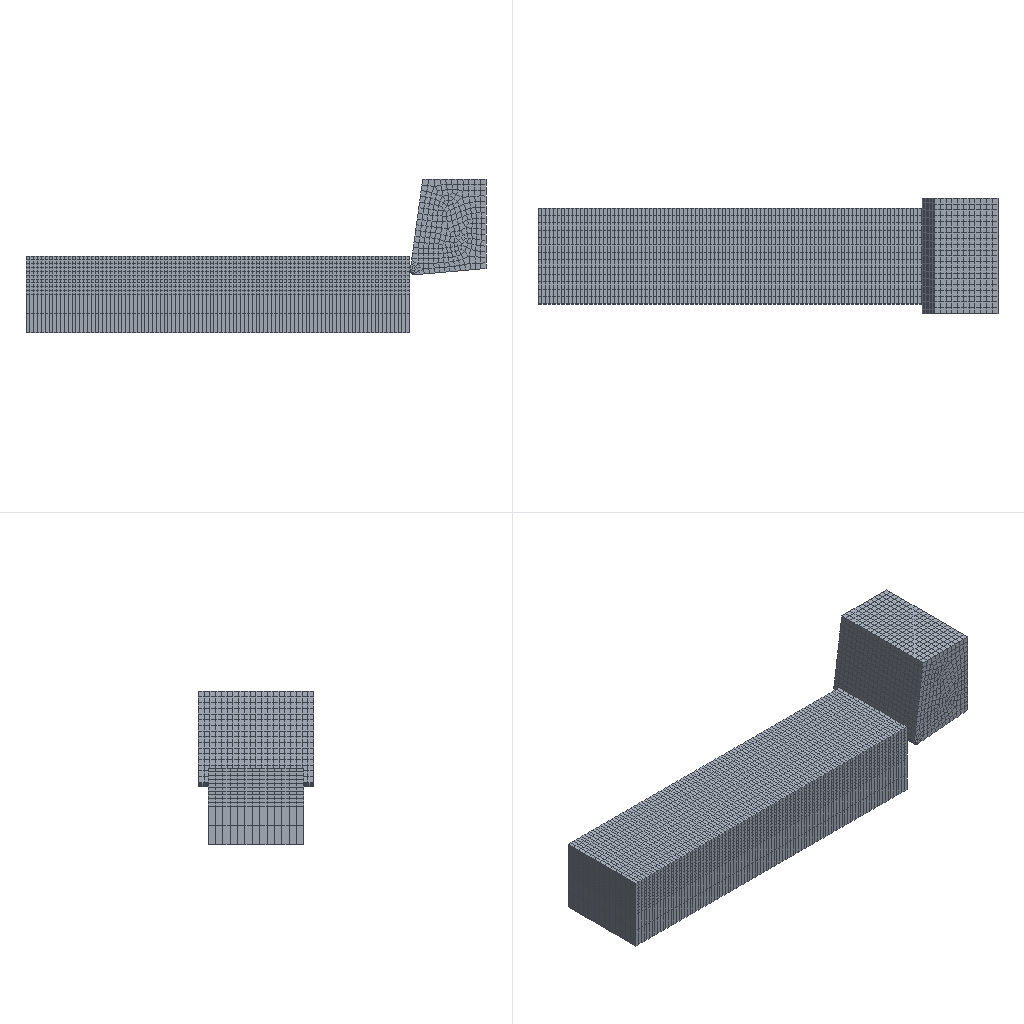Simulation study | abaqus
Set-up summary:
category,name,step,type,value,unit,region
solver,abaqus
solver,version,,,Abaqus/Explicit 2020
units,not stated in the deck,,not stated
analysis,deck,,transient,transient
load_step,Step-1,Step-1,transient
load_step,requested,,,1
mesh,nodes,,,24557
mesh,elements,,,20820
element_type,C3D8R,,solid,20820
load,load commands in deck,,count,1
bc,support commands in deck,,count,7
material,S20MNCR5,,in results
material,S45,,in results
material,TOOL,,in results
check,setup vs results,,match,"per instance, exact: element labels, types and connectivity; labels of the nodes the elements use; coordinates of those nodes at SINGLE_PRECISION in 2 of 2 instance(s)"
Abaqus input file, long lists of numbers shortened:
*Heading
** Job name: Job-1 Model name: Model-1-Copy
** Generated by: Abaqus/CAE 2020
*Preprint, echo=NO, model=NO, history=NO, contact=NO
**
** PARTS
**
*Part, name=tool
*Node
      1,  0.3983, 0.002029,           0.
      2,  0.7735, 0.03465,           0.
** (6172 more lines like these left out)
*Element, type=C3D8R
   1,   66,    3,    4,  275,  360,  297,  298,  569
   2,    5,   24,   69,  274,  299,  318,  363,  568
** (5218 more lines like these left out)
*Node
   6175,  0.4432,          0.5,  0.3
*Nset, nset=tool-RefPt_, internal
6175,
*Nset, nset=Set-8, generate
    1,  6174,     1
*Elset, elset=Set-8, generate
    1,  5220,     1
** Section: tool
*Solid Section, elset=Set-8, material=tool
,
*End Part
**
*Part, name=work
*Node
      1,           0.,           0.,  0.2
      2,           0.,         -0.5,  0.2
** (18380 more lines like these left out)
*Element, type=C3D8R
   1,   278,  1829,  7691,  1037,     1,    17,   941,    48
   2,  1829,  1830,  7692,  7691,    17,    18,   942,   941
** (15598 more lines like these left out)
*Nset, nset=Set-7
     1,     2,     3,     4,     5,     6,     7,     8,    13,    14,    15,    16,    17,    18,    19,    20
    21,    22,    23,    24,    25,    26,    27,    28,    29,    30,    31,    32,    33,    34,    35,    36
** (971 more lines like these left out)
*Elset, elset=Set-7
     1,     2,     3,     4,     5,     6,     7,     8,     9,    10,    11,    12,    13,    14,    15,    16
    17,    18,    19,    20,    21,    22,    23,    24,    25,    26,    27,    28,    29,    30,    31,    32
** (811 more lines like these left out)
*Nset, nset=Set-9
     3,     4,     6,     7,    13,    14,    15,    16,    33,    34,    35,    36,    37,    38,    39,    40
    41,    42,    43,    44,    65,    66,    67,    68,    69,    70,    71,    72,    73,    74,    75,    76
** (529 more lines like these left out)
*Elset, elset=Set-9, generate
  9101,  15600,      1
*Nset, nset=Set-10
     3,     4,     6,     7,    13,    14,    15,    16,    33,    34,    35,    36,    37,    38,    39,    40
    41,    42,    43,    44,    65,    66,    67,    68,    69,    70,    71,    72,    73,    74,    75,    76
** (529 more lines like these left out)
*Elset, elset=Set-10, generate
  9101,  15600,      1
*Nset, nset=Set-11, generate
     1,  18382,      1
*Elset, elset=Set-11, generate
     1,  15600,      1
** Section: work
*Solid Section, elset=Set-11, material=s20mncr5
,
*End Part
**
**
** ASSEMBLY
**
*Assembly, name=Assembly
**
*Instance, name=tool-1, part=tool
       1.625,         0.05,          0.3
       1.625,         0.05,          0.3, 2.625,         0.05,          0.3, 90.
*End Instance
**
*Instance, name=work-1, part=work
*End Instance
**
*Nset, nset=Set-1, instance=work-1
    9,   10,   11,   12,  478,  479,  480,  481,  482,  483,  484,  485,  486,  487,  488,  489
  492,  493,  494,  495,  496,  497,  498,  499,  500,  501,  502,  503,  505,  506,  507,  508
** (87 more lines like these left out)
*Elset, elset=Set-1, instance=work-1
 6514, 6515, 6516, 6517, 6518, 6519, 6520, 6521, 6522, 6523, 6524, 6525, 6526, 6540, 6541, 6542
 6543, 6544, 6545, 6546, 6547, 6548, 6549, 6550, 6551, 6552, 6566, 6567, 6568, 6569, 6570, 6571
** (80 more lines like these left out)
*Nset, nset=Set-2, instance=tool-1
 6175,
*Nset, nset=Set-4, instance=tool-1
    2,    7,    8,   40,   41,   42,   43,   44,   45,   46,   47,   48,   49,   50,   51,   52
   53,   54,   55,   56,   57,   58,   59,   60,   61,   62,   63,   64,  296,  301,  302,  334
** (35 more lines like these left out)
*Nset, nset=Set-4, instance=work-1
     1,     2,     3,     4,     5,     6,     7,     8,     9,    10,    11,    12,    13,    14,    15,    16
    17,    18,    19,    20,    21,    22,    23,    24,    25,    26,    27,    28,    29,    30,    31,    32
** (1059 more lines like these left out)
*Elset, elset=Set-4, instance=tool-1
   24,   25,   29,   33,   34,   35,   37,   39,   41,   43,   44,   46,   47,   49,   50,   51
   52,   53,   54,   70,   73,   81,   86,   88,  100,  101,  285,  286,  290,  294,  295,  296
** (31 more lines like these left out)
*Elset, elset=Set-4, instance=work-1, generate
     1,  15600,      1
*Nset, nset=Set-12, instance=work-1
    9,   10,   11,   12,  478,  479,  480,  481,  482,  483,  484,  485,  486,  487,  488,  489
  492,  493,  494,  495,  496,  497,  498,  499,  500,  501,  502,  503,  505,  506,  507,  508
** (87 more lines like these left out)
*Elset, elset=Set-12, instance=work-1
 6514, 6515, 6516, 6517, 6518, 6519, 6520, 6521, 6522, 6523, 6524, 6525, 6526, 6540, 6541, 6542
 6543, 6544, 6545, 6546, 6547, 6548, 6549, 6550, 6551, 6552, 6566, 6567, 6568, 6569, 6570, 6571
** (80 more lines like these left out)
*Nset, nset=b_Set-12, instance=tool-1, generate
    1,  6174,     1
*Elset, elset=b_Set-12, instance=tool-1, generate
    1,  5220,     1
*Nset, nset=s_Set-9, instance=work-1
     3,     4,     6,     7,    13,    14,    15,    16,    33,    34,    35,    36,    37,    38,    39,    40
    41,    42,    43,    44,    65,    66,    67,    68,    69,    70,    71,    72,    73,    74,    75,    76
** (529 more lines like these left out)
*Elset, elset=s_Set-9, instance=work-1, generate
  9101,  15600,      1
*Nset, nset=s_Set-10, instance=work-1
     1,     2,     3,     4,     5,     6,     7,     8,    13,    14,    15,    16,    17,    18,    19,    20
    21,    22,    23,    24,    25,    26,    27,    28,    29,    30,    31,    32,    33,    34,    35,    36
** (971 more lines like these left out)
*Elset, elset=s_Set-10, instance=work-1
     1,     2,     3,     4,     5,     6,     7,     8,     9,    10,    11,    12,    13,    14,    15,    16
    17,    18,    19,    20,    21,    22,    23,    24,    25,    26,    27,    28,    29,    30,    31,    32
** (892 more lines like these left out)
*Nset, nset=s_Set-11, instance=work-1
     1,     2,     3,     4,     5,     6,     7,     8,    13,    14,    15,    16,    17,    18,    19,    20
    21,    22,    23,    24,    25,    26,    27,    28,    29,    30,    31,    32,    33,    34,    35,    36
** (971 more lines like these left out)
*Elset, elset=s_Set-11, instance=work-1
     1,     2,     3,     4,     5,     6,     7,     8,     9,    10,    11,    12,    13,    14,    15,    16
    17,    18,    19,    20,    21,    22,    23,    24,    25,    26,    27,    28,    29,    30,    31,    32
** (811 more lines like these left out)
*Nset, nset=_PickedSet13, internal, instance=tool-1
 6175,
*Elset, elset=_Surf-4_S5, internal, instance=work-1
  9153,  9154,  9155,  9156,  9157,  9158,  9159,  9160,  9161,  9162,  9163,  9164,  9165,  9218,  9219,  9220
  9221,  9222,  9223,  9224,  9225,  9226,  9227,  9228,  9229,  9230,  9283,  9284,  9285,  9286,  9287,  9288
** (80 more lines like these left out)
*Surface, type=ELEMENT, name=Surf-4
_Surf-4_S5, S5
*Elset, elset=_m_Surf-1_S5, internal, instance=tool-1
   29,   33,   34,   39,   44,   86,  100,  290,  294,  295,  300,  305,  347,  361,  551,  555
  556,  561,  566,  608,  622,  812,  816,  817,  822,  827,  869,  883, 1073, 1077, 1078, 1083
** (7 more lines like these left out)
*Elset, elset=_m_Surf-1_S3, internal, instance=tool-1
   37,   41,   43,   88,  298,  302,  304,  349,  559,  563,  565,  610,  820,  824,  826,  871
 1081, 1085, 1087, 1132, 1342, 1346, 1348, 1393, 1603, 1607, 1609, 1654, 1864, 1868, 1870, 1915
** (3 more lines like these left out)
*Elset, elset=_m_Surf-1_S6, internal, instance=tool-1
   46,   49,   51,   52,   53,   70,   81,  101,  307,  310,  312,  313,  314,  331,  342,  362
  568,  571,  573,  574,  575,  592,  603,  623,  829,  832,  834,  835,  836,  853,  864,  884
** (8 more lines like these left out)
*Elset, elset=_m_Surf-1_S4, internal, instance=tool-1
   24,   25,   34,   35,   47,   50,   54,   73,  285,  286,  295,  296,  308,  311,  315,  334
  546,  547,  556,  557,  569,  572,  576,  595,  807,  808,  817,  818,  830,  833,  837,  856
** (8 more lines like these left out)
*Surface, type=ELEMENT, name=m_Surf-1
_m_Surf-1_S5, S5
_m_Surf-1_S3, S3
_m_Surf-1_S6, S6
_m_Surf-1_S4, S4
*Elset, elset=_m_Surf-3_S5, internal, instance=tool-1
   29,   33,   34,   39,   44,   86,  100,  290,  294,  295,  300,  305,  347,  361,  551,  555
  556,  561,  566,  608,  622,  812,  816,  817,  822,  827,  869,  883, 1073, 1077, 1078, 1083
** (7 more lines like these left out)
*Elset, elset=_m_Surf-3_S3, internal, instance=tool-1
   37,   41,   43,   88,  298,  302,  304,  349,  559,  563,  565,  610,  820,  824,  826,  871
 1081, 1085, 1087, 1132, 1342, 1346, 1348, 1393, 1603, 1607, 1609, 1654, 1864, 1868, 1870, 1915
** (3 more lines like these left out)
*Elset, elset=_m_Surf-3_S6, internal, instance=tool-1
   46,   49,   51,   52,   53,   70,   81,  101,  307,  310,  312,  313,  314,  331,  342,  362
  568,  571,  573,  574,  575,  592,  603,  623,  829,  832,  834,  835,  836,  853,  864,  884
** (8 more lines like these left out)
*Elset, elset=_m_Surf-3_S4, internal, instance=tool-1
   24,   25,   34,   35,   47,   50,   54,   73,  285,  286,  295,  296,  308,  311,  315,  334
  546,  547,  556,  557,  569,  572,  576,  595,  807,  808,  817,  818,  830,  833,  837,  856
** (8 more lines like these left out)
*Surface, type=ELEMENT, name=m_Surf-3
_m_Surf-3_S5, S5
_m_Surf-3_S3, S3
_m_Surf-3_S6, S6
_m_Surf-3_S4, S4
*Elset, elset=_m_Surf-5_S4, internal, instance=tool-1
    1,    3,   13,   14,   15,   16,   17,   18,   20,   23,   24,   25,   26,   31,   34,   35
   44,   47,   50,   54,   55,   56,   65,   67,   73,   82,   83,   84,  255,  262,  264,  274
** (35 more lines like these left out)
*Elset, elset=_m_Surf-5_S3, internal, instance=tool-1
    2,   37,   41,   43,   58,   60,   88,  263,  298,  302,  304,  319,  321,  349,  524,  559
  563,  565,  580,  582,  610,  785,  820,  824,  826,  841,  843,  871, 1046, 1081, 1085, 1087
** (7 more lines like these left out)
*Elset, elset=_m_Surf-5_S6, internal, instance=tool-1
    5,    6,   10,   22,   30,   32,   33,   45,   46,   49,   51,   52,   53,   61,   62,   63
   68,   70,   71,   81,  101,  266,  267,  271,  283,  291,  293,  294,  306,  307,  310,  312
** (25 more lines like these left out)
*Elset, elset=_m_Surf-5_S5, internal, instance=tool-1
   29,   33,   34,   39,   44,   86,  100,  290,  294,  295,  300,  305,  347,  361,  551,  555
  556,  561,  566,  608,  622,  812,  816,  817,  822,  827,  869,  883, 1073, 1077, 1078, 1083
** (7 more lines like these left out)
*Elset, elset=_m_Surf-5_S2, internal, instance=tool-1, generate
 4960,  5220,     1
*Elset, elset=_m_Surf-5_S1, internal, instance=tool-1, generate
   1,  261,    1
*Surface, type=ELEMENT, name=m_Surf-5
_m_Surf-5_S4, S4
_m_Surf-5_S3, S3
_m_Surf-5_S6, S6
_m_Surf-5_S2, S2
_m_Surf-5_S5, S5
_m_Surf-5_S1, S1
*Surface, type=NODE, name=s_Set-11_CNS_, internal
s_Set-11, 1.
** Constraint: Constraint-1
*Rigid Body, ref node=_PickedSet13, elset=b_Set-12
*End Assembly
**
** MATERIALS
**
*Material, name=s20mncr5
*Damage Initiation, criterion=SHEAR
 1.5,0.,0.
*Damage Evolution, type=DISPLACEMENT
 0.001,
*Density
 8.24e-09,
*Elastic
200000., 0.3
*Expansion
 1.3e-05,
*Plastic
1200.,0.
*Material, name=s45
*Conductivity
 50.2,
*Density
 7.8e-09,
*Elastic
210000., 0.3
*Expansion
 1.5e-05,
*Plastic, hardening=JOHNSON COOK
507., 320., 0.28, 1.06,1538.,  25.
*Rate Dependent, type=JOHNSON COOK
 0.064,1.
*Specific Heat
 5e+08,
*Material, name=tool
*Conductivity
120.,
*Density
 1.57e-08,
*Elastic
650000., 0.22
*Expansion
 5.2e-06,
*Specific Heat
 3.43e+08,
**
** INTERACTION PROPERTIES
**
*Surface Interaction, name=IntProp-1
*Friction
 0.2,
*Surface Behavior, pressure-overclosure=HARD
*Surface Interaction, name=chip
*Friction
 0.5,
*Surface Behavior, pressure-overclosure=HARD
**
** BOUNDARY CONDITIONS
**
** Name: BC-1 Type: 对称/反对称/完全固定
*Boundary
Set-12, ENCASTRE
** ----------------------------------------------------------------
**
** STEP: Step-1
**
*Step, name=Step-1, nlgeom=YES
*Dynamic, Explicit
, 0.0004
*Bulk Viscosity
0.06, 1.2
** Mass Scaling: Semi-Automatic
**               Whole Model
*Fixed Mass Scaling, factor=50.
**
** BOUNDARY CONDITIONS
**
** Name: [REDACTED] : Velocity/Angular velocity
*Boundary, type=VELOCITY
Set-2, 1, 1, -5000.
Set-2, 2, 2
Set-2, 3, 3
Set-2, 4, 4
Set-2, 5, 5
Set-2, 6, 6
**
** INTERACTIONS
**
** Interaction: Int-1
*Contact Pair, interaction=IntProp-1, mechanical constraint=KINEMATIC, cpset=Int-1
m_Surf-5, s_Set-11_CNS_
** Interaction: Int-2
*Contact Pair, interaction=chip, mechanical constraint=KINEMATIC, cpset=Int-2
Surf-4,
**
** OUTPUT REQUESTS
**
*Restart, write, number interval=1, time marks=NO
**
** FIELD OUTPUT: F-Output-1
**
*Output, field, number interval=50
*Node Output
A, CF, RF, RM, RT, U, V
*Element Output, directions=YES
E, EVF, LE, MISES, MISESMAX, PE, PEEQ, PEEQMAX, PEEQT, PEEQVAVG, PEMAG, PEVAVG, S, SF, STATUS, SVAVG
*Contact Output
CDISP, CSTRESS
**
** HISTORY OUTPUT: H-Output-1
**
*Output, history, time interval=8e-08
*Node Output, nset=Set-2
RF1, RF2, RF3
*End Step
Results summary:
result,step,Step-1,completed,increments=50810 time=0.0004/0.0004
result,analysis,,,transient
result,last_loadstep,,,1
result,primary field,,,U
result,reaction total,,FX,2.52,model units
result,reaction total,,FY,-5.188,model units
result,reaction total,,FZ,3.279,model units